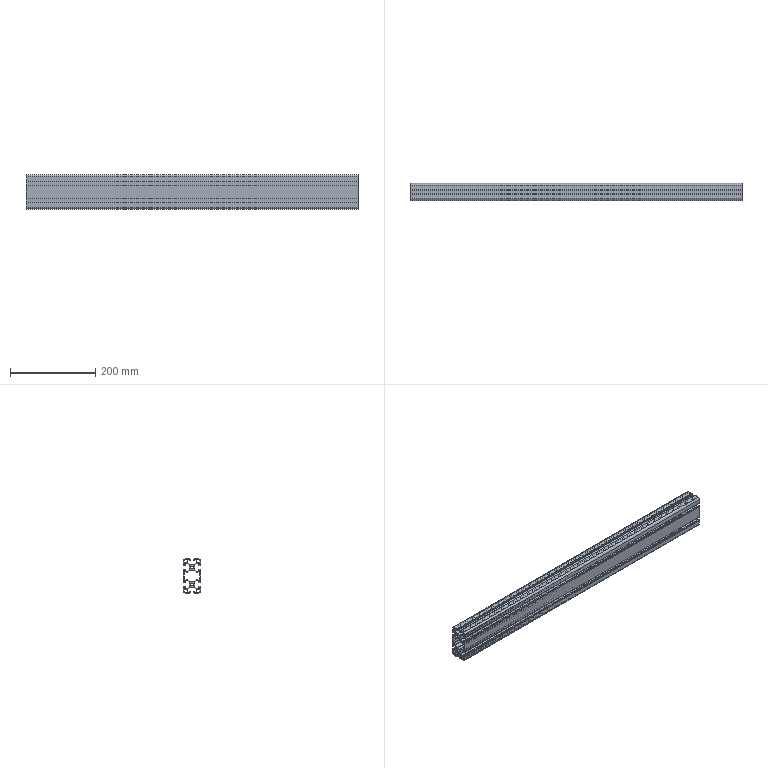Part | STEP file | MK-8-4080H-L-02 profile 4080H standard type 735mm | 1 solid | 294 faces | box 779 x 40 x 80 mm | volume 632330 mm3 | cylinder 148 | plane 142 | cone 4 | commonest cylinder face diameters 0.6 x44 2 x44 4 x28 0.4 x14 6 x4 6.8 x4